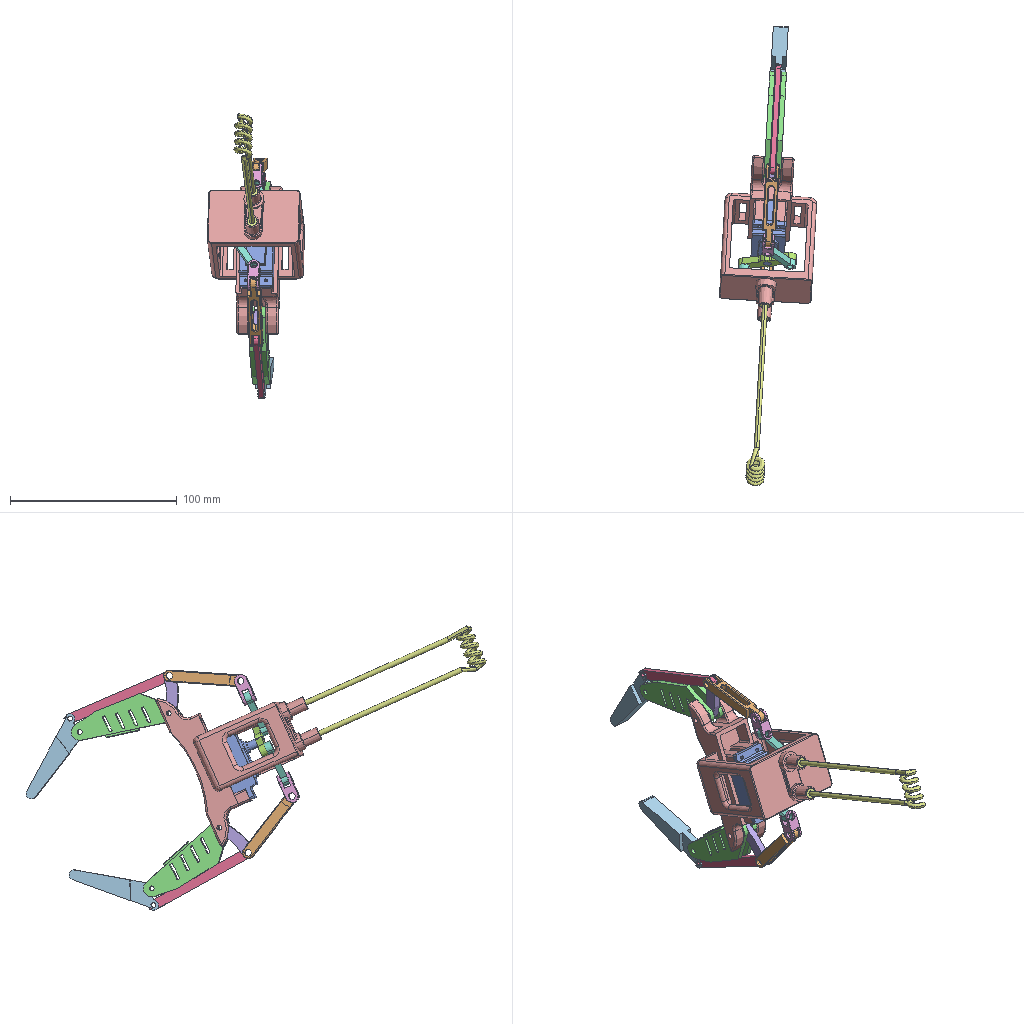Assembly | SolidWorks | 11 different items | 18 placed | box 58 x 276 x 170 mm
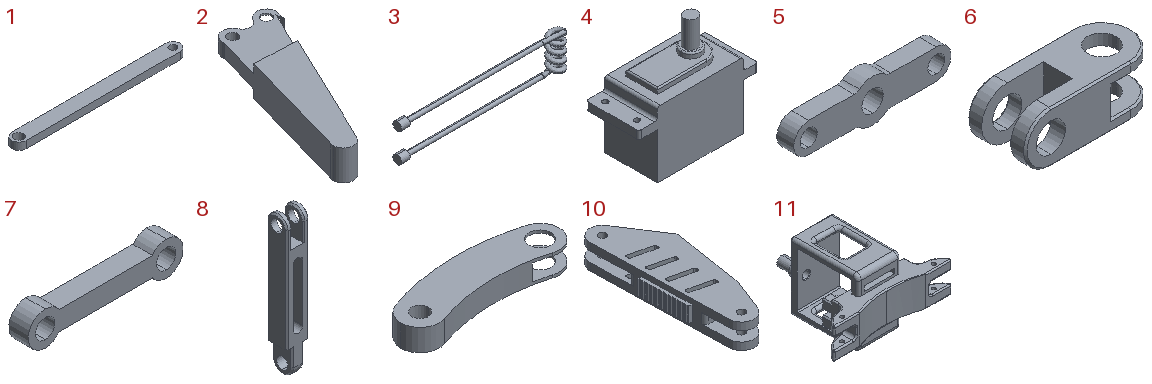Parts list (item | quantity | size | volume | features):
1 | x2 | 71 x 6 x 3 mm | 1196 mm3 | features Extrusion 1, Scale 1
2 | x2 | 28.674 x 51.63 x 9 mm | 3668 mm3 | features ICE 2, Extrusion 1, MirrorPattern 1, Scale 1
3 | x1 | 115.5 x 11 x 27.126 mm | 2602 mm3 | features Blend 2, ICE 2, Fillet 1, Helix 1, Sweep 1
4 | x1 | 45 x 20 x 39 mm | 17798 mm3 | features ICE 6, Fillet 2, Extrusion 1, Scale 1
5 | x1 | 37 x 4 x 10 mm | 874.953 mm3 | features Extrusion 1, Scale 1
6 | x2 | 18.5 x 8 x 7 mm | 447.364 mm3 | features ICE 3, Chamfer 1, Extrusion 1, Scale 1
7 | x2 | 32 x 4 x 7 mm | 501.781 mm3 | features Extrusion 1, Scale 1
8 | x2 | 8 x 7 x 50 mm | 1532 mm3 | features ICE 3, Chamfer 1, Extrusion 1, Scale 1
9 | x2 | 29.5 x 9.079 x 4 mm | 609.677 mm3 | features Extrusion 1, ICE 1, Scale 1
10 | x2 | 21.607 x 64.987 x 10 mm | 6323 mm3 | features ICE 6, Fillet 2, Extrusion 1, LPattern 1, Scale 1
11 | x1 | 96.57 x 80.995 x 55 mm | 46597 mm3 | features ICE 16, Fillet 10, MirrorPattern 3, Chamfer 2, 3DProfileFeature 1, Extrusion 1, HoleWzd 1, Scale 1
Mates (type | each side: item.copy, entity, surface, feature):
Coincident | 11.1 face plane Cut-Extrude1 | 4.1 face plane Boss-Extrude1 | 2 times
Coincident | 11.1 face plane Boss-Extrude2 | 4.1 face plane Boss-Extrude1
Concentric | 11.1 edge | 9.1 edge
Concentric | 11.1 edge | 9.2 edge
Concentric | 11.1 edge | 10.1 edge
Coincident | 11.1 face plane Cut-Extrude2 | 10.1 face plane Boss-Extrude1
Concentric | 11.1 edge | 10.2 edge
Coincident | 11.1 face plane Cut-Extrude2 | 10.2 face plane Boss-Extrude1
Concentric | 4.1 face cylinder Boss-Extrude4 | 5.1 face cylinder Boss-Extrude1
Coincident | 4.1 face plane Boss-Extrude4 | 5.1 face plane Boss-Extrude1
Concentric | 5.1 edge | 7.1 edge
Coincident | 5.1 face plane Boss-Extrude1 | 7.1 face plane Boss-Extrude1
Concentric | 5.1 edge | 7.2 edge
Coincident | 5.1 face plane Boss-Extrude1 | 7.2 face plane Boss-Extrude1
Concentric | 6.1 edge | 7.1 edge
Coincident | 6.1 face plane Cut-Extrude3 | 7.1 edge
Concentric | 6.1 edge | 8.1 edge
Coincident | 6.1 face plane Cut-Extrude1 | 8.1 face plane Boss-Extrude1
Concentric | 6.2 edge | 7.2 edge
Coincident | 6.2 face plane Cut-Extrude3 | 7.2 face plane Boss-Extrude1
Concentric | 6.2 edge | 8.2 edge
Coincident | 6.2 face plane Cut-Extrude1 | 8.2 face plane Boss-Extrude1
Concentric | 8.1 edge | 9.1 edge
Coincident | 8.1 face plane Boss-Extrude1 | 9.1 face plane Boss-Extrude1
Concentric | 8.1 edge | 1.1 edge
Concentric | 8.2 edge | 9.2 edge
Coincident | 8.2 face plane Boss-Extrude1 | 9.2 face plane Boss-Extrude1
Coincident | 9.1 face plane Boss-Extrude1 | 10.2 face plane Cut-Extrude1
Coincident | 9.1 face plane Cut-Extrude1 | 1.1 face plane Boss-Extrude1
Coincident | 9.2 face plane Boss-Extrude1 | 10.1 face plane Cut-Extrude1
Concentric | 9.2 edge | 1.2 edge
Coincident | 9.2 face plane Cut-Extrude1 | 1.2 face plane Boss-Extrude1
Concentric | 10.1 edge | 2.1 edge
Coincident | 10.1 face plane Cut-Extrude1 | 2.1 face plane Boss-Extrude1
Concentric | 10.2 face cylinder Boss-Extrude1 | 2.2 face cylinder Boss-Extrude1
Coincident | 10.2 face plane Cut-Extrude1 | 2.2 face plane Boss-Extrude1
Concentric | 1.2 edge | 2.1 edge
Concentric | 1.1 edge | 2.2 edge
Concentric | 11.1 face cylinder Boss-Extrude9 | 3.1 face cylinder Boss-Extrude1 | 2 times
Coincident | 11.1 face plane Boss-Extrude9 | 3.1 face plane Boss-Extrude2